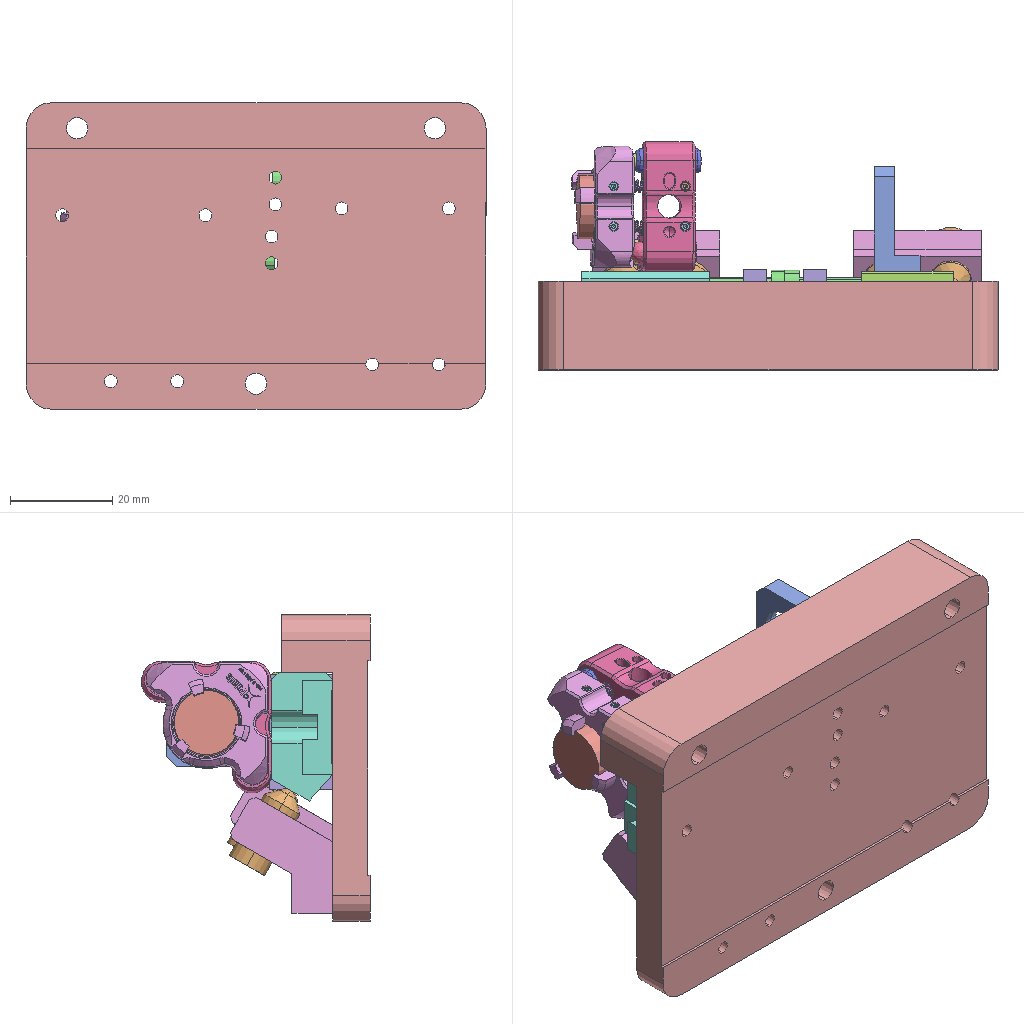Assembly | SolidWorks | 10 different items | 16 placed | box 90 x 45 x 60 mm
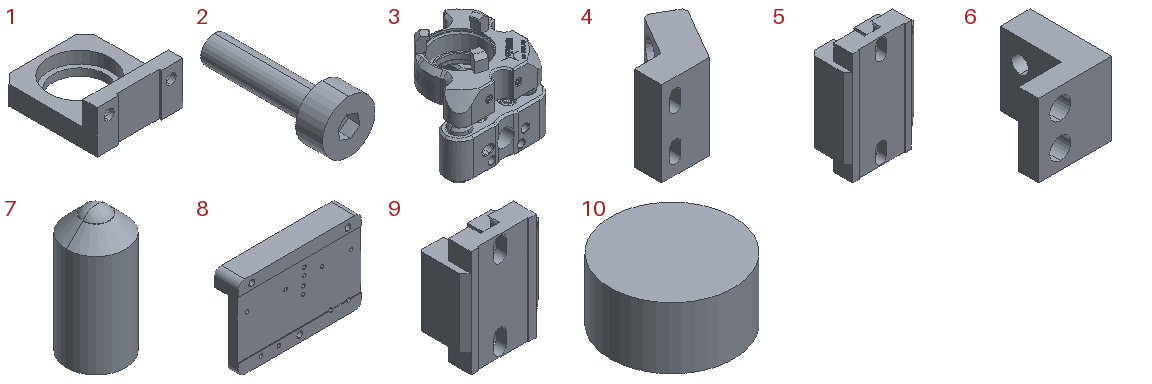Parts list (item | quantity | size | volume | features):
1 | x1 | 18 x 20.5 x 9 mm | 1150 mm3 | features MoveFace 4, ICE 2, BaseBody 1, Chamfer 1, DelFace 1, HoleWzd 1
2 | x2 | 5.86 x 15 x 5.86 mm | 160.113 mm3 | features ICE 2, Extrusion 1
3 | x1 | 25.4 x 25.4 x 24.471 mm | 4593 mm3 | features BaseBody 27
4 | x2 | 22.618 x 20.004 x 25 mm | 4524 mm3 | features ICE 15, MoveFace 2, Chamfer 1, Extrusion 1
5 | x1 | 25.164 x 12 x 35 mm | 7043 mm3 | features ICE 10, Chamfer 1, DelFace 1, Extrusion 1, MoveFace 1
6 | x2 | 11 x 12.3 x 11 mm | 750.231 mm3 | features ICE 2, Chamfer 1, Extrusion 1, HoleWzd 1
7 | x4 | 8 x 8 x 17 mm | 759.813 mm3 | features Chamfer 1, Extrusion 1, Revolution 1
8 | x1 | 90 x 17.28 x 60 mm | 45456 mm3 | features ICE 4, HoleWzd 2, Extrusion 1, Fillet 1
9 | x1 | 23.18 x 12 x 28 mm | 4754 mm3 | features ICE 10, MoveFace 3, Chamfer 2, DelFace 2, Extrusion 1, HoleWzd 1
10 | x1 | 12.7 x 12.7 x 6.35 mm | 804.398 mm3 | features Extrusion 1
Mates (type | each side: item.copy, entity, surface, feature):
Coincident | 8.1 face plane Boss-Extrude1 | 9.1 face plane Boss-Extrude1
Coincident | 8.1 face plane Boss-Extrude2 | 9.1 face plane Cut-Extrude8
Coincident | 1.1 face plane Input 1 | 9.1 face plane Boss-Extrude1
Concentric | 1.1 face cylinder Hole Size (per %) Socket Head Cap Screw Type 2 | 9.1 face cylinder Cut-Extrude11 | 2 times
Slot | 8.1 face cylinder M3 Tapped Hole1 | 9.1 face plane Cut-Extrude12 | 2 times
Coincident | 8.1 face plane Boss-Extrude1 | 4.1 face plane Cut-Extrude13
Coincident | 8.1 face plane Boss-Extrude1 | 4.2 face plane Cut-Extrude13
Slot | 4.1 face plane Cut-Extrude17 | 8.1 face cylinder M3 Tapped Hole1
Slot | 8.1 face cylinder M3 Tapped Hole1 | 4.1 face plane Cut-Extrude17
Slot | 8.1 face cylinder M3 Tapped Hole1 | 4.2 face plane Cut-Extrude17 | 2 times
Coincident | 8.1 face plane Boss-Extrude1 | 5.1 face plane Boss-Extrude1
Slot | 5.1 face plane Cut-Extrude12 | 8.1 face cylinder M3 Tapped Hole1 | 2 times
Concentric | 4.1 face cylinder Cut-Extrude2 | 7.1 face cylinder Boss-Extrude1
Concentric | 4.1 face cylinder Cut-Extrude2 | 7.2 face cylinder Boss-Extrude1
Concentric | 4.2 face cylinder Cut-Extrude2 | 7.3 face cylinder Boss-Extrude1
Tangent | 5.1 face plane Cut-Extrude1 | 7.2 face sphere Revolve2
Tangent | 5.1 face plane Cut-Extrude1 | 7.1 face sphere Revolve2
Tangent | 9.1 face plane Cut-Extrude1 | 7.3 face sphere Revolve2
Tangent | 9.1 face plane Cut-Extrude1 | 7.4 face sphere Revolve2
Concentric | 4.2 face cylinder Cut-Extrude2 | 7.4 face cylinder Boss-Extrude1
Coincident | 8.1 face plane Boss-Extrude1 | 6.1 face plane Boss-Extrude1
Coincident | 8.1 face plane Boss-Extrude1 | 6.2 face plane Boss-Extrude1
Concentric | 8.1 face cylinder M3 Tapped Hole3 | 6.1 face cylinder Cut-Extrude1 | 2 times
Concentric | 8.1 face cylinder M3 Tapped Hole3 | 6.2 face cylinder Cut-Extrude1 | 2 times
Concentric | 6.1 face cylinder M3 Tapped Hole1 | 2.1 face cylinder Boss-Extrude2
Coincident | 9.1 face plane Boss-Extrude1 | 2.1 face plane Boss-Extrude2
Concentric | 6.2 face cylinder M3 Tapped Hole1 | 2.2 face cylinder Boss-Extrude2
Coincident | 5.1 face plane Boss-Extrude1 | 2.2 face plane Boss-Extrude2
Coincident | 5.1 face plane Boss-Extrude1 | 3.1 face plane Input 23
Concentric | 5.1 face cylinder Cut-Extrude10 | 3.1 face cylinder Input 23
Concentric | 3.1 face cylinder Input 18 | 10.1 face cylinder Boss-Extrude1
Coincident | 3.1 face plane Input 18 | 10.1 face plane Boss-Extrude1